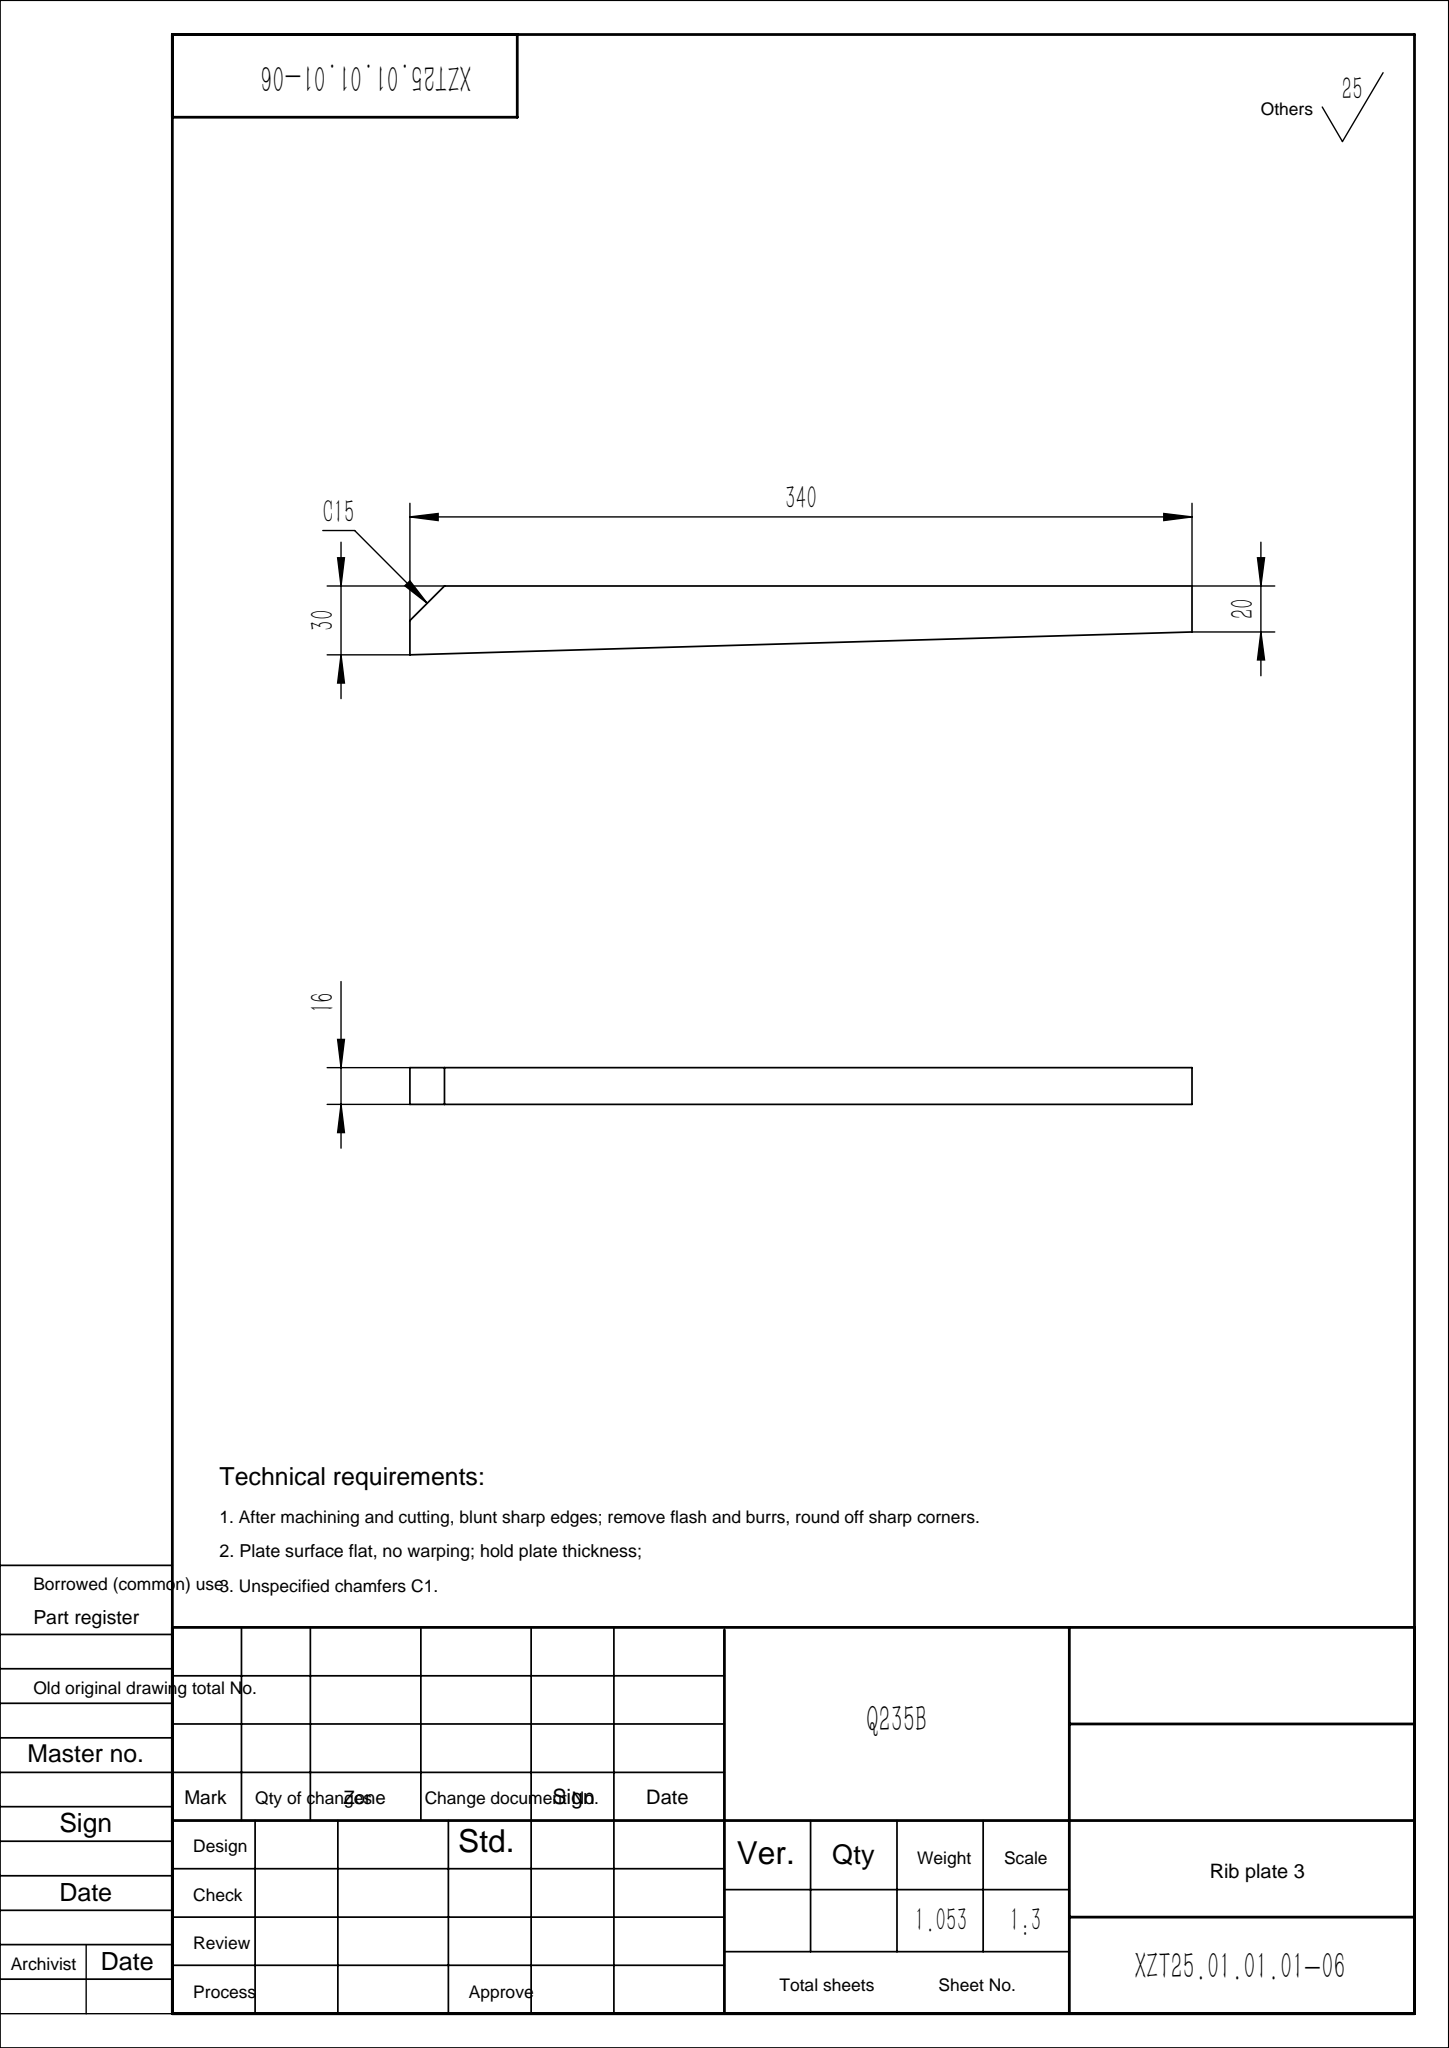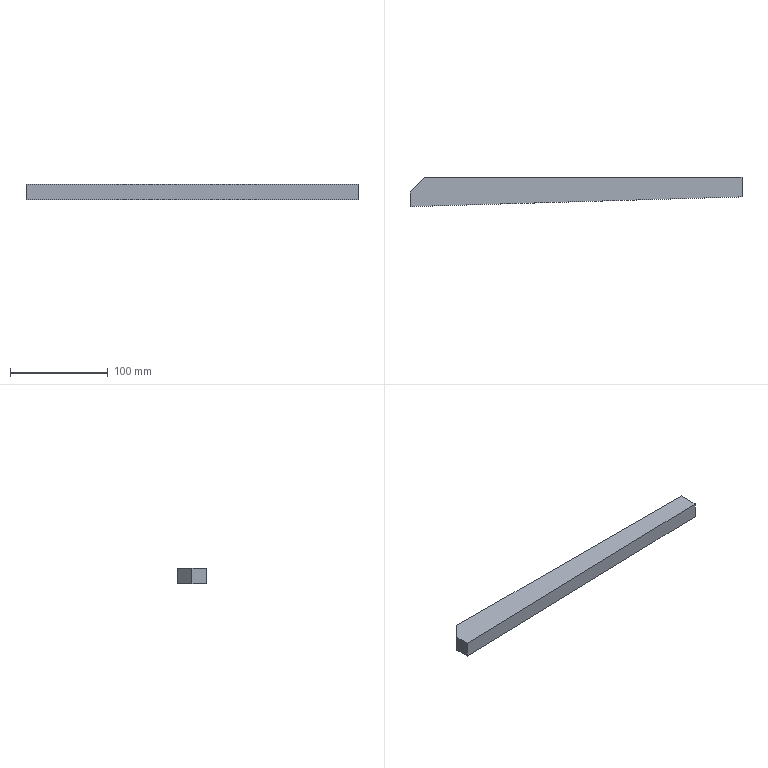Part | SolidWorks | features Chamfer 1, Extrusion 1 | 1 solid | 7 faces | box 340 x 30 x 16 mm | volume 134200 mm3 | plane 7
STEP:
#1=CARTESIAN_POINT('',(0.,0.,-8.));
#2=VERTEX_POINT('',#1);
#3=CARTESIAN_POINT('',(340.,10.,-8.));
#4=VERTEX_POINT('',#3);
#5=CARTESIAN_POINT('',(340.,10.,-8.));
#6=DIRECTION('',(0.9996,0.0294,0.));
#7=VECTOR('',#6,1000.);
#8=LINE('',#5,#7);
#9=EDGE_CURVE('',#2,#4,#8,.T.);
#10=ORIENTED_EDGE('',*,*,#9,.T.);
#11=CARTESIAN_POINT('',(340.,10.,8.));
#12=VERTEX_POINT('',#11);
#13=CARTESIAN_POINT('',(340.,10.,8.));
#14=DIRECTION('',(0.,0.,-1.));
#15=VECTOR('',#14,1000.);
#16=LINE('',#13,#15);
#17=EDGE_CURVE('',#12,#4,#16,.T.);
#18=ORIENTED_EDGE('',*,*,#17,.F.);
#19=CARTESIAN_POINT('',(0.,0.,8.));
#20=VERTEX_POINT('',#19);
#21=CARTESIAN_POINT('',(340.,10.,8.));
#22=DIRECTION('',(0.9996,0.0294,0.));
#23=VECTOR('',#22,1000.);
#24=LINE('',#21,#23);
#25=EDGE_CURVE('',#20,#12,#24,.T.);
#26=ORIENTED_EDGE('',*,*,#25,.F.);
#27=CARTESIAN_POINT('',(0.,0.,8.));
#28=DIRECTION('',(0.,0.,-1.));
#29=VECTOR('',#28,1000.);
#30=LINE('',#27,#29);
#31=EDGE_CURVE('',#20,#2,#30,.T.);
#32=ORIENTED_EDGE('',*,*,#31,.T.);
#33=EDGE_LOOP('',(#10,#18,#26,#32));
#34=FACE_OUTER_BOUND('',#33,.T.);
#35=CARTESIAN_POINT('',(340.,10.,8.));
#36=DIRECTION('',(-0.0294,0.9996,0.));
#37=DIRECTION('',(-0.9996,-0.0294,0.));
#38=AXIS2_PLACEMENT_3D('',#35,#36,#37);
#39=PLANE('',#38);
#40=ADVANCED_FACE('',(#34),#39,.F.);
#41=CARTESIAN_POINT('',(340.,30.,-8.));
#42=VERTEX_POINT('',#41);
#43=CARTESIAN_POINT('',(340.,30.,-8.));
#44=DIRECTION('',(0.,1.,0.));
#45=VECTOR('',#44,1000.);
#46=LINE('',#43,#45);
#47=EDGE_CURVE('',#4,#42,#46,.T.);
#48=ORIENTED_EDGE('',*,*,#47,.T.);
#49=CARTESIAN_POINT('',(340.,30.,8.));
#50=VERTEX_POINT('',#49);
#51=CARTESIAN_POINT('',(340.,30.,8.));
#52=DIRECTION('',(0.,0.,-1.));
#53=VECTOR('',#52,1000.);
#54=LINE('',#51,#53);
#55=EDGE_CURVE('',#50,#42,#54,.T.);
#56=ORIENTED_EDGE('',*,*,#55,.F.);
#57=CARTESIAN_POINT('',(340.,30.,8.));
#58=DIRECTION('',(0.,1.,0.));
#59=VECTOR('',#58,1000.);
#60=LINE('',#57,#59);
#61=EDGE_CURVE('',#12,#50,#60,.T.);
#62=ORIENTED_EDGE('',*,*,#61,.F.);
#63=ORIENTED_EDGE('',*,*,#17,.T.);
#64=EDGE_LOOP('',(#48,#56,#62,#63));
#65=FACE_OUTER_BOUND('',#64,.T.);
#66=CARTESIAN_POINT('',(340.,30.,8.));
#67=DIRECTION('',(-1.,0.,0.));
#68=DIRECTION('',(0.,0.,1.));
#69=AXIS2_PLACEMENT_3D('',#66,#67,#68);
#70=PLANE('',#69);
#71=ADVANCED_FACE('',(#65),#70,.F.);
#72=CARTESIAN_POINT('',(15.,30.,-8.));
#73=VERTEX_POINT('',#72);
#74=CARTESIAN_POINT('',(0.,30.,-8.));
#75=DIRECTION('',(-1.,0.,0.));
#76=VECTOR('',#75,1000.);
#77=LINE('',#74,#76);
#78=EDGE_CURVE('',#42,#73,#77,.T.);
#79=ORIENTED_EDGE('',*,*,#78,.T.);
#80=CARTESIAN_POINT('',(15.,30.,8.));
#81=VERTEX_POINT('',#80);
#82=CARTESIAN_POINT('',(15.,30.,8.));
#83=DIRECTION('',(0.,0.,1.));
#84=VECTOR('',#83,1000.);
#85=LINE('',#82,#84);
#86=EDGE_CURVE('',#73,#81,#85,.T.);
#87=ORIENTED_EDGE('',*,*,#86,.T.);
#88=CARTESIAN_POINT('',(0.,30.,8.));
#89=DIRECTION('',(-1.,0.,0.));
#90=VECTOR('',#89,1000.);
#91=LINE('',#88,#90);
#92=EDGE_CURVE('',#50,#81,#91,.T.);
#93=ORIENTED_EDGE('',*,*,#92,.F.);
#94=ORIENTED_EDGE('',*,*,#55,.T.);
#95=EDGE_LOOP('',(#79,#87,#93,#94));
#96=FACE_OUTER_BOUND('',#95,.T.);
#97=CARTESIAN_POINT('',(0.,30.,8.));
#98=DIRECTION('',(0.,-1.,0.));
#99=DIRECTION('',(0.,0.,-1.));
#100=AXIS2_PLACEMENT_3D('',#97,#98,#99);
#101=PLANE('',#100);
#102=ADVANCED_FACE('',(#96),#101,.F.);
#103=CARTESIAN_POINT('',(0.,15.,8.));
#104=VERTEX_POINT('',#103);
#105=CARTESIAN_POINT('',(0.,0.,8.));
#106=DIRECTION('',(0.,-1.,0.));
#107=VECTOR('',#106,1000.);
#108=LINE('',#105,#107);
#109=EDGE_CURVE('',#104,#20,#108,.T.);
#110=ORIENTED_EDGE('',*,*,#109,.F.);
#111=CARTESIAN_POINT('',(0.,15.,-8.));
#112=VERTEX_POINT('',#111);
#113=CARTESIAN_POINT('',(0.,15.,8.));
#114=DIRECTION('',(0.,0.,-1.));
#115=VECTOR('',#114,1000.);
#116=LINE('',#113,#115);
#117=EDGE_CURVE('',#104,#112,#116,.T.);
#118=ORIENTED_EDGE('',*,*,#117,.T.);
#119=CARTESIAN_POINT('',(0.,0.,-8.));
#120=DIRECTION('',(0.,-1.,0.));
#121=VECTOR('',#120,1000.);
#122=LINE('',#119,#121);
#123=EDGE_CURVE('',#112,#2,#122,.T.);
#124=ORIENTED_EDGE('',*,*,#123,.T.);
#125=ORIENTED_EDGE('',*,*,#31,.F.);
#126=EDGE_LOOP('',(#110,#118,#124,#125));
#127=FACE_OUTER_BOUND('',#126,.T.);
#128=CARTESIAN_POINT('',(0.,0.,8.));
#129=DIRECTION('',(1.,0.,0.));
#130=DIRECTION('',(0.,0.,-1.));
#131=AXIS2_PLACEMENT_3D('',#128,#129,#130);
#132=PLANE('',#131);
#133=ADVANCED_FACE('',(#127),#132,.F.);
#134=ORIENTED_EDGE('',*,*,#92,.T.);
#135=CARTESIAN_POINT('',(0.,15.,8.));
#136=DIRECTION('',(-0.7071,-0.7071,0.));
#137=VECTOR('',#136,1000.);
#138=LINE('',#135,#137);
#139=EDGE_CURVE('',#81,#104,#138,.T.);
#140=ORIENTED_EDGE('',*,*,#139,.T.);
#141=ORIENTED_EDGE('',*,*,#109,.T.);
#142=ORIENTED_EDGE('',*,*,#25,.T.);
#143=ORIENTED_EDGE('',*,*,#61,.T.);
#144=EDGE_LOOP('',(#134,#140,#141,#142,#143));
#145=FACE_OUTER_BOUND('',#144,.T.);
#146=CARTESIAN_POINT('',(0.,0.,8.));
#147=DIRECTION('',(0.,0.,-1.));
#148=DIRECTION('',(-1.,0.,0.));
#149=AXIS2_PLACEMENT_3D('',#146,#147,#148);
#150=PLANE('',#149);
#151=ADVANCED_FACE('',(#145),#150,.F.);
#152=ORIENTED_EDGE('',*,*,#123,.F.);
#153=CARTESIAN_POINT('',(-7.5,7.5,-8.));
#154=DIRECTION('',(0.7071,0.7071,0.));
#155=VECTOR('',#154,1000.);
#156=LINE('',#153,#155);
#157=EDGE_CURVE('',#112,#73,#156,.T.);
#158=ORIENTED_EDGE('',*,*,#157,.T.);
#159=ORIENTED_EDGE('',*,*,#78,.F.);
#160=ORIENTED_EDGE('',*,*,#47,.F.);
#161=ORIENTED_EDGE('',*,*,#9,.F.);
#162=EDGE_LOOP('',(#152,#158,#159,#160,#161));
#163=FACE_OUTER_BOUND('',#162,.T.);
#164=CARTESIAN_POINT('',(0.,0.,-8.));
#165=DIRECTION('',(0.,0.,-1.));
#166=DIRECTION('',(-1.,0.,0.));
#167=AXIS2_PLACEMENT_3D('',#164,#165,#166);
#168=PLANE('',#167);
#169=ADVANCED_FACE('',(#163),#168,.T.);
#170=ORIENTED_EDGE('',*,*,#139,.F.);
#171=ORIENTED_EDGE('',*,*,#86,.F.);
#172=ORIENTED_EDGE('',*,*,#157,.F.);
#173=ORIENTED_EDGE('',*,*,#117,.F.);
#174=EDGE_LOOP('',(#170,#171,#172,#173));
#175=FACE_OUTER_BOUND('',#174,.T.);
#176=CARTESIAN_POINT('',(0.,15.,8.));
#177=DIRECTION('',(0.7071,-0.7071,0.));
#178=DIRECTION('',(0.,0.,-1.));
#179=AXIS2_PLACEMENT_3D('',#176,#177,#178);
#180=PLANE('',#179);
#181=ADVANCED_FACE('',(#175),#180,.F.);
#182=CLOSED_SHELL('',(#40,#71,#102,#133,#151,#169,#181));
#183=MANIFOLD_SOLID_BREP('',#182);
#184=CARTESIAN_POINT('',(0.,0.,0.));
#185=DIRECTION('',(0.,0.,1.));
#186=DIRECTION('',(1.,0.,0.));
#187=AXIS2_PLACEMENT_3D('',#184,#185,#186);
#188=(LENGTH_UNIT()NAMED_UNIT(*)SI_UNIT(.MILLI.,.METRE.));
#189=UNCERTAINTY_MEASURE_WITH_UNIT(LENGTH_MEASURE(0.00001),#188,'','');
#190=(NAMED_UNIT(*)PLANE_ANGLE_UNIT()SI_UNIT($,.RADIAN.));
#191=(NAMED_UNIT(*)SI_UNIT($,.STERADIAN.)SOLID_ANGLE_UNIT());
#192=(GEOMETRIC_REPRESENTATION_CONTEXT(3)GLOBAL_UNCERTAINTY_ASSIGNED_CONTEXT((#189))GLOBAL_UNIT_ASSIGNED_CONTEXT((#188,#190,#191))REPRESENTATION_CONTEXT('',''));
#193=ADVANCED_BREP_SHAPE_REPRESENTATION('',(#183,#187),#192);